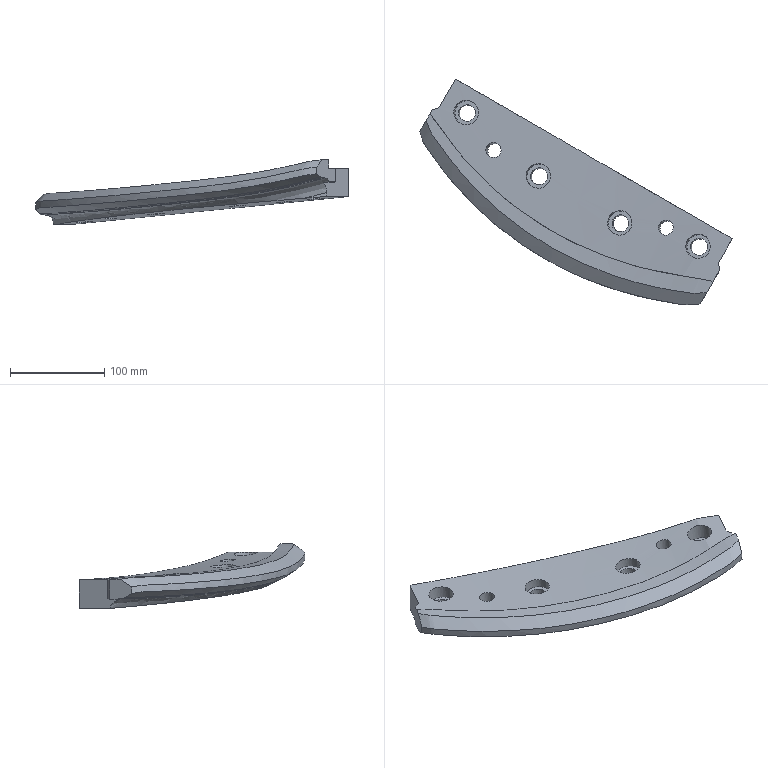Part | NX | features solid 2 | 1 solid | 35 faces | box 331.31 x 239.465 x 68.79 mm | volume 810873 mm3 | plane 15 | spline 10 | cylinder 10 | commonest cylinder face diameters 18 x4 26 x4 16 x2